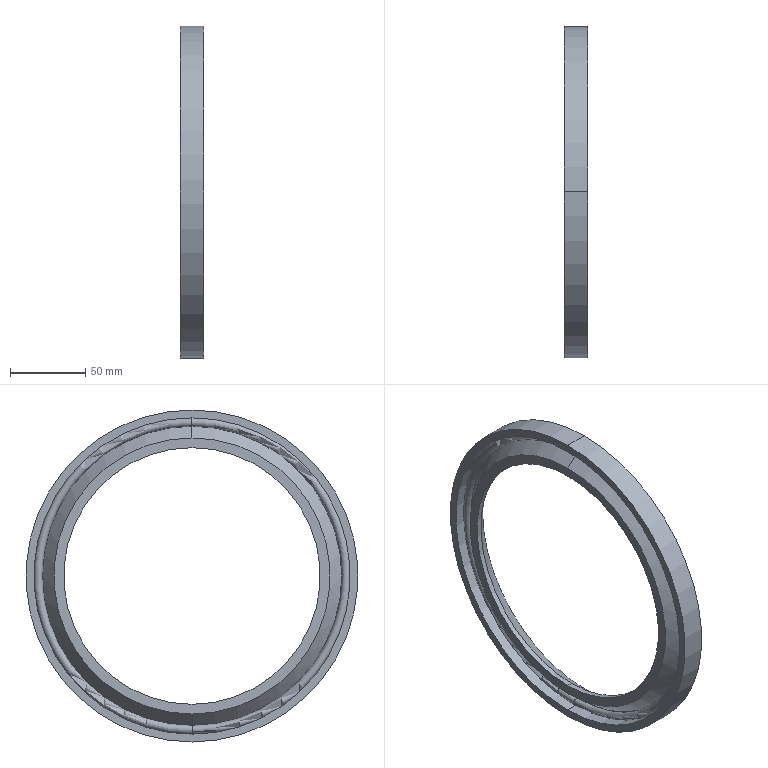Part | STEP file | Seal ring | 2 solids | 19 faces | box 15.499 x 219.997 x 219.997 mm | volume 158146 mm3 | torus 6 | cylinder 6 | cone 4 | plane 3 | commonest cylinder face diameters 170.01 x2 209.598 x2 219.997 x2
STEP:
#1=CARTESIAN_POINT('',(0.,0.,0.));
#2=DIRECTION('',(0.,0.,1.));
#3=DIRECTION('',(1.,0.,0.));
#4=AXIS2_PLACEMENT_3D('',#1,#2,#3);
#5=CARTESIAN_POINT('',(14.065,0.,104.799));
#6=VERTEX_POINT('',#5);
#7=CARTESIAN_POINT('',(14.065,0.,99.229));
#8=VERTEX_POINT('',#7);
#9=CARTESIAN_POINT('',(14.065,0.,102.014));
#10=DIRECTION('',(0.,1.,0.));
#11=DIRECTION('',(0.,0.,1.));
#12=AXIS2_PLACEMENT_3D('',#9,#10,#11);
#13=CIRCLE('',#12,2.785);
#14=CARTESIAN_POINT('',(14.065,0.,0.));
#15=DIRECTION('',(1.,0.,0.));
#16=DIRECTION('',(0.,0.,-1.));
#17=AXIS2_PLACEMENT_3D('',#14,#15,#16);
#18=TOROIDAL_SURFACE('',#17,102.014,2.785);
#19=CARTESIAN_POINT('',(3.142,0.));
#20=DIRECTION('',(0.,1.));
#21=VECTOR('',#20,1.);
#22=LINE('',#19,#21);
#23=(GEOMETRIC_REPRESENTATION_CONTEXT(2)PARAMETRIC_REPRESENTATION_CONTEXT()REPRESENTATION_CONTEXT('',''));
#24=DEFINITIONAL_REPRESENTATION('',(#22),#23);
#25=PCURVE('',#18,#24);
#26=CARTESIAN_POINT('',(14.065,0.,0.));
#27=DIRECTION('',(1.,0.,0.));
#28=DIRECTION('',(0.,0.,-1.));
#29=AXIS2_PLACEMENT_3D('',#26,#27,#28);
#30=TOROIDAL_SURFACE('',#29,102.014,2.785);
#31=CARTESIAN_POINT('',(3.142,0.));
#32=DIRECTION('',(0.,1.));
#33=VECTOR('',#32,1.);
#34=LINE('',#31,#33);
#35=(GEOMETRIC_REPRESENTATION_CONTEXT(2)PARAMETRIC_REPRESENTATION_CONTEXT()REPRESENTATION_CONTEXT('',''));
#36=DEFINITIONAL_REPRESENTATION('',(#34),#35);
#37=PCURVE('',#30,#36);
#38=SURFACE_CURVE('',#13,(#25,#37),.PCURVE_S1.);
#39=EDGE_CURVE('',#6,#8,#38,.T.);
#40=ORIENTED_EDGE('',*,*,#39,.F.);
#41=CARTESIAN_POINT('',(14.065,0.,-104.799));
#42=VERTEX_POINT('',#41);
#43=CARTESIAN_POINT('',(14.065,0.,0.));
#44=DIRECTION('',(1.,0.,0.));
#45=DIRECTION('',(0.,0.,-1.));
#46=AXIS2_PLACEMENT_3D('',#43,#44,#45);
#47=CIRCLE('',#46,104.799);
#48=CARTESIAN_POINT('',(0.,0.));
#49=DIRECTION('',(1.,0.));
#50=VECTOR('',#49,1.);
#51=LINE('',#48,#50);
#52=(GEOMETRIC_REPRESENTATION_CONTEXT(2)PARAMETRIC_REPRESENTATION_CONTEXT()REPRESENTATION_CONTEXT('',''));
#53=DEFINITIONAL_REPRESENTATION('',(#51),#52);
#54=PCURVE('',#18,#53);
#55=CARTESIAN_POINT('',(14.065,0.,0.));
#56=DIRECTION('',(1.,0.,0.));
#57=DIRECTION('',(0.,0.,-1.));
#58=AXIS2_PLACEMENT_3D('',#55,#56,#57);
#59=TOROIDAL_SURFACE('',#58,102.014,2.785);
#60=CARTESIAN_POINT('',(0.,6.283));
#61=DIRECTION('',(1.,0.));
#62=VECTOR('',#61,1.);
#63=LINE('',#60,#62);
#64=(GEOMETRIC_REPRESENTATION_CONTEXT(2)PARAMETRIC_REPRESENTATION_CONTEXT()REPRESENTATION_CONTEXT('',''));
#65=DEFINITIONAL_REPRESENTATION('',(#63),#64);
#66=PCURVE('',#59,#65);
#67=SURFACE_CURVE('',#47,(#54,#66),.PCURVE_S1.);
#68=EDGE_CURVE('',#6,#42,#67,.T.);
#69=ORIENTED_EDGE('',*,*,#68,.T.);
#70=CARTESIAN_POINT('',(14.065,0.,-99.229));
#71=VERTEX_POINT('',#70);
#72=CARTESIAN_POINT('',(14.065,0.,-102.014));
#73=DIRECTION('',(0.,-1.,0.));
#74=DIRECTION('',(0.,0.,-1.));
#75=AXIS2_PLACEMENT_3D('',#72,#73,#74);
#76=CIRCLE('',#75,2.785);
#77=CARTESIAN_POINT('',(6.283,0.));
#78=DIRECTION('',(0.,1.));
#79=VECTOR('',#78,1.);
#80=LINE('',#77,#79);
#81=(GEOMETRIC_REPRESENTATION_CONTEXT(2)PARAMETRIC_REPRESENTATION_CONTEXT()REPRESENTATION_CONTEXT('',''));
#82=DEFINITIONAL_REPRESENTATION('',(#80),#81);
#83=PCURVE('',#18,#82);
#84=CARTESIAN_POINT('',(0.,0.));
#85=DIRECTION('',(0.,1.));
#86=VECTOR('',#85,1.);
#87=LINE('',#84,#86);
#88=(GEOMETRIC_REPRESENTATION_CONTEXT(2)PARAMETRIC_REPRESENTATION_CONTEXT()REPRESENTATION_CONTEXT('',''));
#89=DEFINITIONAL_REPRESENTATION('',(#87),#88);
#90=PCURVE('',#30,#89);
#91=SURFACE_CURVE('',#76,(#83,#90),.PCURVE_S1.);
#92=EDGE_CURVE('',#42,#71,#91,.T.);
#93=ORIENTED_EDGE('',*,*,#92,.T.);
#94=CARTESIAN_POINT('',(14.065,0.,0.));
#95=DIRECTION('',(1.,0.,0.));
#96=DIRECTION('',(0.,0.,-1.));
#97=AXIS2_PLACEMENT_3D('',#94,#95,#96);
#98=CIRCLE('',#97,99.229);
#99=CARTESIAN_POINT('',(0.,3.142));
#100=DIRECTION('',(1.,0.));
#101=VECTOR('',#100,1.);
#102=LINE('',#99,#101);
#103=(GEOMETRIC_REPRESENTATION_CONTEXT(2)PARAMETRIC_REPRESENTATION_CONTEXT()REPRESENTATION_CONTEXT('',''));
#104=DEFINITIONAL_REPRESENTATION('',(#102),#103);
#105=PCURVE('',#18,#104);
#106=CARTESIAN_POINT('',(0.,3.142));
#107=DIRECTION('',(1.,0.));
#108=VECTOR('',#107,1.);
#109=LINE('',#106,#108);
#110=(GEOMETRIC_REPRESENTATION_CONTEXT(2)PARAMETRIC_REPRESENTATION_CONTEXT()REPRESENTATION_CONTEXT('',''));
#111=DEFINITIONAL_REPRESENTATION('',(#109),#110);
#112=PCURVE('',#59,#111);
#113=SURFACE_CURVE('',#98,(#105,#112),.PCURVE_S1.);
#114=EDGE_CURVE('',#8,#71,#113,.T.);
#115=ORIENTED_EDGE('',*,*,#114,.F.);
#116=EDGE_LOOP('',(#40,#69,#93,#115));
#117=FACE_BOUND('',#116,.T.);
#118=ADVANCED_FACE('',(#117),#18,.T.);
#119=ORIENTED_EDGE('',*,*,#92,.F.);
#120=CARTESIAN_POINT('',(14.065,0.,0.));
#121=DIRECTION('',(1.,0.,0.));
#122=DIRECTION('',(0.,0.,-1.));
#123=AXIS2_PLACEMENT_3D('',#120,#121,#122);
#124=CIRCLE('',#123,104.799);
#125=CARTESIAN_POINT('',(0.,0.));
#126=DIRECTION('',(1.,0.));
#127=VECTOR('',#126,1.);
#128=LINE('',#125,#127);
#129=(GEOMETRIC_REPRESENTATION_CONTEXT(2)PARAMETRIC_REPRESENTATION_CONTEXT()REPRESENTATION_CONTEXT('',''));
#130=DEFINITIONAL_REPRESENTATION('',(#128),#129);
#131=PCURVE('',#30,#130);
#132=CARTESIAN_POINT('',(14.065,0.,0.));
#133=DIRECTION('',(1.,0.,0.));
#134=DIRECTION('',(0.,0.,-1.));
#135=AXIS2_PLACEMENT_3D('',#132,#133,#134);
#136=TOROIDAL_SURFACE('',#135,102.014,2.785);
#137=CARTESIAN_POINT('',(0.,6.283));
#138=DIRECTION('',(1.,0.));
#139=VECTOR('',#138,1.);
#140=LINE('',#137,#139);
#141=(GEOMETRIC_REPRESENTATION_CONTEXT(2)PARAMETRIC_REPRESENTATION_CONTEXT()REPRESENTATION_CONTEXT('',''));
#142=DEFINITIONAL_REPRESENTATION('',(#140),#141);
#143=PCURVE('',#136,#142);
#144=SURFACE_CURVE('',#124,(#131,#143),.PCURVE_S1.);
#145=EDGE_CURVE('',#42,#6,#144,.T.);
#146=ORIENTED_EDGE('',*,*,#145,.T.);
#147=ORIENTED_EDGE('',*,*,#39,.T.);
#148=CARTESIAN_POINT('',(14.065,0.,0.));
#149=DIRECTION('',(1.,0.,0.));
#150=DIRECTION('',(0.,0.,-1.));
#151=AXIS2_PLACEMENT_3D('',#148,#149,#150);
#152=CIRCLE('',#151,99.229);
#153=CARTESIAN_POINT('',(0.,3.142));
#154=DIRECTION('',(1.,0.));
#155=VECTOR('',#154,1.);
#156=LINE('',#153,#155);
#157=(GEOMETRIC_REPRESENTATION_CONTEXT(2)PARAMETRIC_REPRESENTATION_CONTEXT()REPRESENTATION_CONTEXT('',''));
#158=DEFINITIONAL_REPRESENTATION('',(#156),#157);
#159=PCURVE('',#30,#158);
#160=CARTESIAN_POINT('',(0.,3.142));
#161=DIRECTION('',(1.,0.));
#162=VECTOR('',#161,1.);
#163=LINE('',#160,#162);
#164=(GEOMETRIC_REPRESENTATION_CONTEXT(2)PARAMETRIC_REPRESENTATION_CONTEXT()REPRESENTATION_CONTEXT('',''));
#165=DEFINITIONAL_REPRESENTATION('',(#163),#164);
#166=PCURVE('',#136,#165);
#167=SURFACE_CURVE('',#152,(#159,#166),.PCURVE_S1.);
#168=EDGE_CURVE('',#71,#8,#167,.T.);
#169=ORIENTED_EDGE('',*,*,#168,.F.);
#170=EDGE_LOOP('',(#119,#146,#147,#169));
#171=FACE_BOUND('',#170,.T.);
#172=ADVANCED_FACE('',(#171),#30,.T.);
#173=ORIENTED_EDGE('',*,*,#145,.F.);
#174=CARTESIAN_POINT('',(14.065,0.,-102.014));
#175=DIRECTION('',(0.,-1.,0.));
#176=DIRECTION('',(0.,0.,-1.));
#177=AXIS2_PLACEMENT_3D('',#174,#175,#176);
#178=CIRCLE('',#177,2.785);
#179=CARTESIAN_POINT('',(0.,0.));
#180=DIRECTION('',(0.,1.));
#181=VECTOR('',#180,1.);
#182=LINE('',#179,#181);
#183=(GEOMETRIC_REPRESENTATION_CONTEXT(2)PARAMETRIC_REPRESENTATION_CONTEXT()REPRESENTATION_CONTEXT('',''));
#184=DEFINITIONAL_REPRESENTATION('',(#182),#183);
#185=PCURVE('',#136,#184);
#186=CARTESIAN_POINT('',(6.283,0.));
#187=DIRECTION('',(0.,1.));
#188=VECTOR('',#187,1.);
#189=LINE('',#186,#188);
#190=(GEOMETRIC_REPRESENTATION_CONTEXT(2)PARAMETRIC_REPRESENTATION_CONTEXT()REPRESENTATION_CONTEXT('',''));
#191=DEFINITIONAL_REPRESENTATION('',(#189),#190);
#192=PCURVE('',#59,#191);
#193=SURFACE_CURVE('',#178,(#185,#192),.PCURVE_S1.);
#194=EDGE_CURVE('',#71,#42,#193,.T.);
#195=ORIENTED_EDGE('',*,*,#194,.F.);
#196=ORIENTED_EDGE('',*,*,#168,.T.);
#197=CARTESIAN_POINT('',(14.065,0.,102.014));
#198=DIRECTION('',(0.,1.,0.));
#199=DIRECTION('',(0.,0.,1.));
#200=AXIS2_PLACEMENT_3D('',#197,#198,#199);
#201=CIRCLE('',#200,2.785);
#202=CARTESIAN_POINT('',(3.142,0.));
#203=DIRECTION('',(0.,1.));
#204=VECTOR('',#203,1.);
#205=LINE('',#202,#204);
#206=(GEOMETRIC_REPRESENTATION_CONTEXT(2)PARAMETRIC_REPRESENTATION_CONTEXT()REPRESENTATION_CONTEXT('',''));
#207=DEFINITIONAL_REPRESENTATION('',(#205),#206);
#208=PCURVE('',#136,#207);
#209=CARTESIAN_POINT('',(3.142,0.));
#210=DIRECTION('',(0.,1.));
#211=VECTOR('',#210,1.);
#212=LINE('',#209,#211);
#213=(GEOMETRIC_REPRESENTATION_CONTEXT(2)PARAMETRIC_REPRESENTATION_CONTEXT()REPRESENTATION_CONTEXT('',''));
#214=DEFINITIONAL_REPRESENTATION('',(#212),#213);
#215=PCURVE('',#59,#214);
#216=SURFACE_CURVE('',#201,(#208,#215),.PCURVE_S1.);
#217=EDGE_CURVE('',#8,#6,#216,.T.);
#218=ORIENTED_EDGE('',*,*,#217,.T.);
#219=EDGE_LOOP('',(#173,#195,#196,#218));
#220=FACE_BOUND('',#219,.T.);
#221=ADVANCED_FACE('',(#220),#136,.T.);
#222=ORIENTED_EDGE('',*,*,#68,.F.);
#223=ORIENTED_EDGE('',*,*,#217,.F.);
#224=ORIENTED_EDGE('',*,*,#114,.T.);
#225=ORIENTED_EDGE('',*,*,#194,.T.);
#226=EDGE_LOOP('',(#222,#223,#224,#225));
#227=FACE_BOUND('',#226,.T.);
#228=ADVANCED_FACE('',(#227),#59,.T.);
#229=CLOSED_SHELL('',(#118,#172,#221,#228));
#230=MANIFOLD_SOLID_BREP('',#229);
#231=CARTESIAN_POINT('',(5.58,0.,-104.799));
#232=VERTEX_POINT('',#231);
#233=CARTESIAN_POINT('',(14.065,0.,-104.799));
#234=VERTEX_POINT('',#233);
#235=CARTESIAN_POINT('',(0.,0.,-104.799));
#236=DIRECTION('',(1.,0.,0.));
#237=VECTOR('',#236,1.);
#238=LINE('',#235,#237);
#239=CARTESIAN_POINT('',(0.,0.,0.));
#240=DIRECTION('',(1.,0.,0.));
#241=DIRECTION('',(0.,0.,-1.));
#242=AXIS2_PLACEMENT_3D('',#239,#240,#241);
#243=CYLINDRICAL_SURFACE('',#242,104.799);
#244=CARTESIAN_POINT('',(6.283,0.));
#245=DIRECTION('',(0.,1.));
#246=VECTOR('',#245,1.);
#247=LINE('',#244,#246);
#248=(GEOMETRIC_REPRESENTATION_CONTEXT(2)PARAMETRIC_REPRESENTATION_CONTEXT()REPRESENTATION_CONTEXT('',''));
#249=DEFINITIONAL_REPRESENTATION('',(#247),#248);
#250=PCURVE('',#243,#249);
#251=CARTESIAN_POINT('',(0.,0.,0.));
#252=DIRECTION('',(1.,0.,0.));
#253=DIRECTION('',(0.,0.,-1.));
#254=AXIS2_PLACEMENT_3D('',#251,#252,#253);
#255=CYLINDRICAL_SURFACE('',#254,104.799);
#256=CARTESIAN_POINT('',(0.,0.));
#257=DIRECTION('',(0.,1.));
#258=VECTOR('',#257,1.);
#259=LINE('',#256,#258);
#260=(GEOMETRIC_REPRESENTATION_CONTEXT(2)PARAMETRIC_REPRESENTATION_CONTEXT()REPRESENTATION_CONTEXT('',''));
#261=DEFINITIONAL_REPRESENTATION('',(#259),#260);
#262=PCURVE('',#255,#261);
#263=SURFACE_CURVE('',#238,(#250,#262),.PCURVE_S1.);
#264=EDGE_CURVE('',#232,#234,#263,.T.);
#265=ORIENTED_EDGE('',*,*,#264,.T.);
#266=CARTESIAN_POINT('',(14.065,0.,104.799));
#267=VERTEX_POINT('',#266);
#268=CARTESIAN_POINT('',(14.065,0.,0.));
#269=DIRECTION('',(1.,0.,0.));
#270=DIRECTION('',(0.,0.,-1.));
#271=AXIS2_PLACEMENT_3D('',#268,#269,#270);
#272=CIRCLE('',#271,104.799);
#273=CARTESIAN_POINT('',(0.,14.065));
#274=DIRECTION('',(1.,0.));
#275=VECTOR('',#274,1.);
#276=LINE('',#273,#275);
#277=(GEOMETRIC_REPRESENTATION_CONTEXT(2)PARAMETRIC_REPRESENTATION_CONTEXT()REPRESENTATION_CONTEXT('',''));
#278=DEFINITIONAL_REPRESENTATION('',(#276),#277);
#279=PCURVE('',#243,#278);
#280=CARTESIAN_POINT('',(14.065,0.,0.));
#281=DIRECTION('',(1.,0.,0.));
#282=DIRECTION('',(0.,0.,-1.));
#283=AXIS2_PLACEMENT_3D('',#280,#281,#282);
#284=TOROIDAL_SURFACE('',#283,102.014,2.785);
#285=CARTESIAN_POINT('',(0.,0.));
#286=DIRECTION('',(1.,0.));
#287=VECTOR('',#286,1.);
#288=LINE('',#285,#287);
#289=(GEOMETRIC_REPRESENTATION_CONTEXT(2)PARAMETRIC_REPRESENTATION_CONTEXT()REPRESENTATION_CONTEXT('',''));
#290=DEFINITIONAL_REPRESENTATION('',(#288),#289);
#291=PCURVE('',#284,#290);
#292=SURFACE_CURVE('',#272,(#279,#291),.PCURVE_S1.);
#293=EDGE_CURVE('',#267,#234,#292,.T.);
#294=ORIENTED_EDGE('',*,*,#293,.F.);
#295=CARTESIAN_POINT('',(5.58,0.,104.799));
#296=VERTEX_POINT('',#295);
#297=CARTESIAN_POINT('',(0.,0.,104.799));
#298=DIRECTION('',(1.,0.,0.));
#299=VECTOR('',#298,1.);
#300=LINE('',#297,#299);
#301=CARTESIAN_POINT('',(3.142,0.));
#302=DIRECTION('',(0.,1.));
#303=VECTOR('',#302,1.);
#304=LINE('',#301,#303);
#305=(GEOMETRIC_REPRESENTATION_CONTEXT(2)PARAMETRIC_REPRESENTATION_CONTEXT()REPRESENTATION_CONTEXT('',''));
#306=DEFINITIONAL_REPRESENTATION('',(#304),#305);
#307=PCURVE('',#243,#306);
#308=CARTESIAN_POINT('',(3.142,0.));
#309=DIRECTION('',(0.,1.));
#310=VECTOR('',#309,1.);
#311=LINE('',#308,#310);
#312=(GEOMETRIC_REPRESENTATION_CONTEXT(2)PARAMETRIC_REPRESENTATION_CONTEXT()REPRESENTATION_CONTEXT('',''));
#313=DEFINITIONAL_REPRESENTATION('',(#311),#312);
#314=PCURVE('',#255,#313);
#315=SURFACE_CURVE('',#300,(#307,#314),.PCURVE_S1.);
#316=EDGE_CURVE('',#296,#267,#315,.T.);
#317=ORIENTED_EDGE('',*,*,#316,.F.);
#318=CARTESIAN_POINT('',(5.58,0.,0.));
#319=DIRECTION('',(1.,0.,0.));
#320=DIRECTION('',(0.,0.,-1.));
#321=AXIS2_PLACEMENT_3D('',#318,#319,#320);
#322=CIRCLE('',#321,104.799);
#323=CARTESIAN_POINT('',(0.,5.58));
#324=DIRECTION('',(1.,0.));
#325=VECTOR('',#324,1.);
#326=LINE('',#323,#325);
#327=(GEOMETRIC_REPRESENTATION_CONTEXT(2)PARAMETRIC_REPRESENTATION_CONTEXT()REPRESENTATION_CONTEXT('',''));
#328=DEFINITIONAL_REPRESENTATION('',(#326),#327);
#329=PCURVE('',#243,#328);
#330=CARTESIAN_POINT('',(5.58,0.,0.));
#331=DIRECTION('',(-1.,0.,0.));
#332=DIRECTION('',(0.,0.,1.));
#333=AXIS2_PLACEMENT_3D('',#330,#331,#332);
#334=PLANE('',#333);
#335=CARTESIAN_POINT('',(-104.799,0.));
#336=CARTESIAN_POINT('',(-104.799,181.517));
#337=CARTESIAN_POINT('',(52.399,90.759));
#338=CARTESIAN_POINT('',(209.598,0.));
#339=CARTESIAN_POINT('',(52.399,-90.759));
#340=CARTESIAN_POINT('',(-104.799,-181.517));
#341=CARTESIAN_POINT('',(-104.799,0.));
#342=(BOUNDED_CURVE()B_SPLINE_CURVE(2,(#335,#336,#337,#338,#339,#340,#341),.UNSPECIFIED.,.T.,.F.)B_SPLINE_CURVE_WITH_KNOTS((1,2,2,2,2,1),(-2.094,0.,2.094,4.189,6.283,8.378),.UNSPECIFIED.)CURVE()GEOMETRIC_REPRESENTATION_ITEM()RATIONAL_B_SPLINE_CURVE((1.,0.5,1.,0.5,1.,0.5,1.))REPRESENTATION_ITEM(''));
#343=(GEOMETRIC_REPRESENTATION_CONTEXT(2)PARAMETRIC_REPRESENTATION_CONTEXT()REPRESENTATION_CONTEXT('',''));
#344=DEFINITIONAL_REPRESENTATION('',(#342),#343);
#345=PCURVE('',#334,#344);
#346=SURFACE_CURVE('',#322,(#329,#345),.PCURVE_S1.);
#347=EDGE_CURVE('',#296,#232,#346,.T.);
#348=ORIENTED_EDGE('',*,*,#347,.T.);
#349=EDGE_LOOP('',(#265,#294,#317,#348));
#350=FACE_BOUND('',#349,.F.);
#351=ADVANCED_FACE('',(#350),#243,.F.);
#352=CARTESIAN_POINT('',(5.58,0.,-109.999));
#353=VERTEX_POINT('',#352);
#354=CARTESIAN_POINT('',(5.58,0.,109.999));
#355=VERTEX_POINT('',#354);
#356=CARTESIAN_POINT('',(5.58,0.,0.));
#357=DIRECTION('',(1.,0.,0.));
#358=DIRECTION('',(0.,0.,-1.));
#359=AXIS2_PLACEMENT_3D('',#356,#357,#358);
#360=CIRCLE('',#359,109.999);
#361=CARTESIAN_POINT('',(0.,0.,0.));
#362=DIRECTION('',(1.,0.,0.));
#363=DIRECTION('',(0.,0.,-1.));
#364=AXIS2_PLACEMENT_3D('',#361,#362,#363);
#365=CYLINDRICAL_SURFACE('',#364,109.999);
#366=CARTESIAN_POINT('',(0.,5.58));
#367=DIRECTION('',(1.,0.));
#368=VECTOR('',#367,1.);
#369=LINE('',#366,#368);
#370=(GEOMETRIC_REPRESENTATION_CONTEXT(2)PARAMETRIC_REPRESENTATION_CONTEXT()REPRESENTATION_CONTEXT('',''));
#371=DEFINITIONAL_REPRESENTATION('',(#369),#370);
#372=PCURVE('',#365,#371);
#373=CARTESIAN_POINT('',(-109.999,0.));
#374=CARTESIAN_POINT('',(-109.999,190.523));
#375=CARTESIAN_POINT('',(54.999,95.262));
#376=CARTESIAN_POINT('',(219.997,0.));
#377=CARTESIAN_POINT('',(54.999,-95.262));
#378=CARTESIAN_POINT('',(-109.999,-190.523));
#379=CARTESIAN_POINT('',(-109.999,0.));
#380=(BOUNDED_CURVE()B_SPLINE_CURVE(2,(#373,#374,#375,#376,#377,#378,#379),.UNSPECIFIED.,.T.,.F.)B_SPLINE_CURVE_WITH_KNOTS((1,2,2,2,2,1),(-2.094,0.,2.094,4.189,6.283,8.378),.UNSPECIFIED.)CURVE()GEOMETRIC_REPRESENTATION_ITEM()RATIONAL_B_SPLINE_CURVE((1.,0.5,1.,0.5,1.,0.5,1.))REPRESENTATION_ITEM(''));
#381=(GEOMETRIC_REPRESENTATION_CONTEXT(2)PARAMETRIC_REPRESENTATION_CONTEXT()REPRESENTATION_CONTEXT('',''));
#382=DEFINITIONAL_REPRESENTATION('',(#380),#381);
#383=PCURVE('',#334,#382);
#384=SURFACE_CURVE('',#360,(#372,#383),.PCURVE_S1.);
#385=EDGE_CURVE('',#353,#355,#384,.T.);
#386=ORIENTED_EDGE('',*,*,#385,.T.);
#387=CARTESIAN_POINT('',(21.079,0.,109.999));
#388=VERTEX_POINT('',#387);
#389=CARTESIAN_POINT('',(0.,0.,109.999));
#390=DIRECTION('',(1.,0.,0.));
#391=VECTOR('',#390,1.);
#392=LINE('',#389,#391);
#393=CARTESIAN_POINT('',(3.142,0.));
#394=DIRECTION('',(0.,1.));
#395=VECTOR('',#394,1.);
#396=LINE('',#393,#395);
#397=(GEOMETRIC_REPRESENTATION_CONTEXT(2)PARAMETRIC_REPRESENTATION_CONTEXT()REPRESENTATION_CONTEXT('',''));
#398=DEFINITIONAL_REPRESENTATION('',(#396),#397);
#399=PCURVE('',#365,#398);
#400=CARTESIAN_POINT('',(0.,0.,0.));
#401=DIRECTION('',(1.,0.,0.));
#402=DIRECTION('',(0.,0.,-1.));
#403=AXIS2_PLACEMENT_3D('',#400,#401,#402);
#404=CYLINDRICAL_SURFACE('',#403,109.999);
#405=CARTESIAN_POINT('',(3.142,0.));
#406=DIRECTION('',(0.,1.));
#407=VECTOR('',#406,1.);
#408=LINE('',#405,#407);
#409=(GEOMETRIC_REPRESENTATION_CONTEXT(2)PARAMETRIC_REPRESENTATION_CONTEXT()REPRESENTATION_CONTEXT('',''));
#410=DEFINITIONAL_REPRESENTATION('',(#408),#409);
#411=PCURVE('',#404,#410);
#412=SURFACE_CURVE('',#392,(#399,#411),.PCURVE_S1.);
#413=EDGE_CURVE('',#355,#388,#412,.T.);
#414=ORIENTED_EDGE('',*,*,#413,.T.);
#415=CARTESIAN_POINT('',(21.079,0.,-109.999));
#416=VERTEX_POINT('',#415);
#417=CARTESIAN_POINT('',(21.079,0.,0.));
#418=DIRECTION('',(1.,0.,0.));
#419=DIRECTION('',(0.,0.,-1.));
#420=AXIS2_PLACEMENT_3D('',#417,#418,#419);
#421=CIRCLE('',#420,109.999);
#422=CARTESIAN_POINT('',(0.,21.079));
#423=DIRECTION('',(1.,0.));
#424=VECTOR('',#423,1.);
#425=LINE('',#422,#424);
#426=(GEOMETRIC_REPRESENTATION_CONTEXT(2)PARAMETRIC_REPRESENTATION_CONTEXT()REPRESENTATION_CONTEXT('',''));
#427=DEFINITIONAL_REPRESENTATION('',(#425),#426);
#428=PCURVE('',#365,#427);
#429=CARTESIAN_POINT('',(21.079,0.,0.));
#430=DIRECTION('',(-1.,0.,0.));
#431=DIRECTION('',(0.,0.,1.));
#432=AXIS2_PLACEMENT_3D('',#429,#430,#431);
#433=PLANE('',#432);
#434=CARTESIAN_POINT('',(-109.999,0.));
#435=CARTESIAN_POINT('',(-109.999,190.523));
#436=CARTESIAN_POINT('',(54.999,95.262));
#437=CARTESIAN_POINT('',(219.997,0.));
#438=CARTESIAN_POINT('',(54.999,-95.262));
#439=CARTESIAN_POINT('',(-109.999,-190.523));
#440=CARTESIAN_POINT('',(-109.999,0.));
#441=(BOUNDED_CURVE()B_SPLINE_CURVE(2,(#434,#435,#436,#437,#438,#439,#440),.UNSPECIFIED.,.T.,.F.)B_SPLINE_CURVE_WITH_KNOTS((1,2,2,2,2,1),(-2.094,0.,2.094,4.189,6.283,8.378),.UNSPECIFIED.)CURVE()GEOMETRIC_REPRESENTATION_ITEM()RATIONAL_B_SPLINE_CURVE((1.,0.5,1.,0.5,1.,0.5,1.))REPRESENTATION_ITEM(''));
#442=(GEOMETRIC_REPRESENTATION_CONTEXT(2)PARAMETRIC_REPRESENTATION_CONTEXT()REPRESENTATION_CONTEXT('',''));
#443=DEFINITIONAL_REPRESENTATION('',(#441),#442);
#444=PCURVE('',#433,#443);
#445=SURFACE_CURVE('',#421,(#428,#444),.PCURVE_S1.);
#446=EDGE_CURVE('',#416,#388,#445,.T.);
#447=ORIENTED_EDGE('',*,*,#446,.F.);
#448=CARTESIAN_POINT('',(0.,0.,-109.999));
#449=DIRECTION('',(1.,0.,0.));
#450=VECTOR('',#449,1.);
#451=LINE('',#448,#450);
#452=CARTESIAN_POINT('',(0.,0.));
#453=DIRECTION('',(0.,1.));
#454=VECTOR('',#453,1.);
#455=LINE('',#452,#454);
#456=(GEOMETRIC_REPRESENTATION_CONTEXT(2)PARAMETRIC_REPRESENTATION_CONTEXT()REPRESENTATION_CONTEXT('',''));
#457=DEFINITIONAL_REPRESENTATION('',(#455),#456);
#458=PCURVE('',#365,#457);
#459=CARTESIAN_POINT('',(6.283,0.));
#460=DIRECTION('',(0.,1.));
#461=VECTOR('',#460,1.);
#462=LINE('',#459,#461);
#463=(GEOMETRIC_REPRESENTATION_CONTEXT(2)PARAMETRIC_REPRESENTATION_CONTEXT()REPRESENTATION_CONTEXT('',''));
#464=DEFINITIONAL_REPRESENTATION('',(#462),#463);
#465=PCURVE('',#404,#464);
#466=SURFACE_CURVE('',#451,(#458,#465),.PCURVE_S1.);
#467=EDGE_CURVE('',#353,#416,#466,.T.);
#468=ORIENTED_EDGE('',*,*,#467,.F.);
#469=EDGE_LOOP('',(#386,#414,#447,#468));
#470=FACE_BOUND('',#469,.T.);
#471=ADVANCED_FACE('',(#470),#365,.T.);
#472=CARTESIAN_POINT('',(9.062,0.,-85.005));
#473=VERTEX_POINT('',#472);
#474=CARTESIAN_POINT('',(21.079,0.,-95.297));
#475=VERTEX_POINT('',#474);
#476=CARTESIAN_POINT('',(21.079,0.,-95.297));
#477=DIRECTION('',(0.7595,0.,-0.6505));
#478=VECTOR('',#477,1.);
#479=LINE('',#476,#478);
#480=CARTESIAN_POINT('',(21.079,0.,0.));
#481=DIRECTION('',(1.,0.,0.));
#482=DIRECTION('',(0.,0.,-1.));
#483=AXIS2_PLACEMENT_3D('',#480,#481,#482);
#484=CONICAL_SURFACE('',#483,95.297,0.7082);
#485=CARTESIAN_POINT('',(6.283,0.));
#486=DIRECTION('',(0.,1.));
#487=VECTOR('',#486,1.);
#488=LINE('',#485,#487);
#489=(GEOMETRIC_REPRESENTATION_CONTEXT(2)PARAMETRIC_REPRESENTATION_CONTEXT()REPRESENTATION_CONTEXT('',''));
#490=DEFINITIONAL_REPRESENTATION('',(#488),#489);
#491=PCURVE('',#484,#490);
#492=CARTESIAN_POINT('',(21.079,0.,0.));
#493=DIRECTION('',(1.,0.,0.));
#494=DIRECTION('',(0.,0.,-1.));
#495=AXIS2_PLACEMENT_3D('',#492,#493,#494);
#496=CONICAL_SURFACE('',#495,95.297,0.7082);
#497=CARTESIAN_POINT('',(0.,0.));
#498=DIRECTION('',(0.,1.));
#499=VECTOR('',#498,1.);
#500=LINE('',#497,#499);
#501=(GEOMETRIC_REPRESENTATION_CONTEXT(2)PARAMETRIC_REPRESENTATION_CONTEXT()REPRESENTATION_CONTEXT('',''));
#502=DEFINITIONAL_REPRESENTATION('',(#500),#501);
#503=PCURVE('',#496,#502);
#504=SURFACE_CURVE('',#479,(#491,#503),.PCURVE_S1.);
#505=EDGE_CURVE('',#473,#475,#504,.T.);
#506=ORIENTED_EDGE('',*,*,#505,.T.);
#507=CARTESIAN_POINT('',(21.079,0.,95.297));
#508=VERTEX_POINT('',#507);
#509=CARTESIAN_POINT('',(21.079,0.,0.));
#510=DIRECTION('',(1.,0.,0.));
#511=DIRECTION('',(0.,0.,-1.));
#512=AXIS2_PLACEMENT_3D('',#509,#510,#511);
#513=CIRCLE('',#512,95.297);
#514=CARTESIAN_POINT('',(0.,0.));
#515=DIRECTION('',(1.,0.));
#516=VECTOR('',#515,1.);
#517=LINE('',#514,#516);
#518=(GEOMETRIC_REPRESENTATION_CONTEXT(2)PARAMETRIC_REPRESENTATION_CONTEXT()REPRESENTATION_CONTEXT('',''));
#519=DEFINITIONAL_REPRESENTATION('',(#517),#518);
#520=PCURVE('',#484,#519);
#521=CARTESIAN_POINT('',(-95.297,0.));
#522=CARTESIAN_POINT('',(-95.297,165.059));
#523=CARTESIAN_POINT('',(47.648,82.529));
#524=CARTESIAN_POINT('',(190.594,0.));
#525=CARTESIAN_POINT('',(47.648,-82.529));
#526=CARTESIAN_POINT('',(-95.297,-165.059));
#527=CARTESIAN_POINT('',(-95.297,0.));
#528=(BOUNDED_CURVE()B_SPLINE_CURVE(2,(#521,#522,#523,#524,#525,#526,#527),.UNSPECIFIED.,.T.,.F.)B_SPLINE_CURVE_WITH_KNOTS((1,2,2,2,2,1),(-2.094,0.,2.094,4.189,6.283,8.378),.UNSPECIFIED.)CURVE()GEOMETRIC_REPRESENTATION_ITEM()RATIONAL_B_SPLINE_CURVE((1.,0.5,1.,0.5,1.,0.5,1.))REPRESENTATION_ITEM(''));
#529=(GEOMETRIC_REPRESENTATION_CONTEXT(2)PARAMETRIC_REPRESENTATION_CONTEXT()REPRESENTATION_CONTEXT('',''));
#530=DEFINITIONAL_REPRESENTATION('',(#528),#529);
#531=PCURVE('',#433,#530);
#532=SURFACE_CURVE('',#513,(#520,#531),.PCURVE_S1.);
#533=EDGE_CURVE('',#508,#475,#532,.T.);
#534=ORIENTED_EDGE('',*,*,#533,.F.);
#535=CARTESIAN_POINT('',(9.062,0.,85.005));
#536=VERTEX_POINT('',#535);
#537=CARTESIAN_POINT('',(21.079,0.,95.297));
#538=DIRECTION('',(0.7595,0.,0.6505));
#539=VECTOR('',#538,1.);
#540=LINE('',#537,#539);
#541=CARTESIAN_POINT('',(3.142,0.));
#542=DIRECTION('',(0.,1.));
#543=VECTOR('',#542,1.);
#544=LINE('',#541,#543);
#545=(GEOMETRIC_REPRESENTATION_CONTEXT(2)PARAMETRIC_REPRESENTATION_CONTEXT()REPRESENTATION_CONTEXT('',''));
#546=DEFINITIONAL_REPRESENTATION('',(#544),#545);
#547=PCURVE('',#484,#546);
#548=CARTESIAN_POINT('',(3.142,0.));
#549=DIRECTION('',(0.,1.));
#550=VECTOR('',#549,1.);
#551=LINE('',#548,#550);
#552=(GEOMETRIC_REPRESENTATION_CONTEXT(2)PARAMETRIC_REPRESENTATION_CONTEXT()REPRESENTATION_CONTEXT('',''));
#553=DEFINITIONAL_REPRESENTATION('',(#551),#552);
#554=PCURVE('',#496,#553);
#555=SURFACE_CURVE('',#540,(#547,#554),.PCURVE_S1.);
#556=EDGE_CURVE('',#536,#508,#555,.T.);
#557=ORIENTED_EDGE('',*,*,#556,.F.);
#558=CARTESIAN_POINT('',(9.062,0.,0.));
#559=DIRECTION('',(1.,0.,0.));
#560=DIRECTION('',(0.,0.,-1.));
#561=AXIS2_PLACEMENT_3D('',#558,#559,#560);
#562=CIRCLE('',#561,85.005);
#563=CARTESIAN_POINT('',(0.,-12.017));
#564=DIRECTION('',(1.,0.));
#565=VECTOR('',#564,1.);
#566=LINE('',#563,#565);
#567=(GEOMETRIC_REPRESENTATION_CONTEXT(2)PARAMETRIC_REPRESENTATION_CONTEXT()REPRESENTATION_CONTEXT('',''));
#568=DEFINITIONAL_REPRESENTATION('',(#566),#567);
#569=PCURVE('',#484,#568);
#570=CARTESIAN_POINT('',(0.,0.,0.));
#571=DIRECTION('',(1.,0.,0.));
#572=DIRECTION('',(0.,0.,-1.));
#573=AXIS2_PLACEMENT_3D('',#570,#571,#572);
#574=CYLINDRICAL_SURFACE('',#573,85.005);
#575=CARTESIAN_POINT('',(0.,9.062));
#576=DIRECTION('',(1.,0.));
#577=VECTOR('',#576,1.);
#578=LINE('',#575,#577);
#579=(GEOMETRIC_REPRESENTATION_CONTEXT(2)PARAMETRIC_REPRESENTATION_CONTEXT()REPRESENTATION_CONTEXT('',''));
#580=DEFINITIONAL_REPRESENTATION('',(#578),#579);
#581=PCURVE('',#574,#580);
#582=SURFACE_CURVE('',#562,(#569,#581),.PCURVE_S1.);
#583=EDGE_CURVE('',#536,#473,#582,.T.);
#584=ORIENTED_EDGE('',*,*,#583,.T.);
#585=EDGE_LOOP('',(#506,#534,#557,#584));
#586=FACE_BOUND('',#585,.F.);
#587=ADVANCED_FACE('',(#586),#484,.F.);
#588=CARTESIAN_POINT('',(5.583,0.,-85.005));
#589=VERTEX_POINT('',#588);
#590=CARTESIAN_POINT('',(0.,0.,-85.005));
#591=DIRECTION('',(1.,0.,0.));
#592=VECTOR('',#591,1.);
#593=LINE('',#590,#592);
#594=CARTESIAN_POINT('',(6.283,0.));
#595=DIRECTION('',(0.,1.));
#596=VECTOR('',#595,1.);
#597=LINE('',#594,#596);
#598=(GEOMETRIC_REPRESENTATION_CONTEXT(2)PARAMETRIC_REPRESENTATION_CONTEXT()REPRESENTATION_CONTEXT('',''));
#599=DEFINITIONAL_REPRESENTATION('',(#597),#598);
#600=PCURVE('',#574,#599);
#601=CARTESIAN_POINT('',(0.,0.,0.));
#602=DIRECTION('',(1.,0.,0.));
#603=DIRECTION('',(0.,0.,-1.));
#604=AXIS2_PLACEMENT_3D('',#601,#602,#603);
#605=CYLINDRICAL_SURFACE('',#604,85.005);
#606=CARTESIAN_POINT('',(0.,0.));
#607=DIRECTION('',(0.,1.));
#608=VECTOR('',#607,1.);
#609=LINE('',#606,#608);
#610=(GEOMETRIC_REPRESENTATION_CONTEXT(2)PARAMETRIC_REPRESENTATION_CONTEXT()REPRESENTATION_CONTEXT('',''));
#611=DEFINITIONAL_REPRESENTATION('',(#609),#610);
#612=PCURVE('',#605,#611);
#613=SURFACE_CURVE('',#593,(#600,#612),.PCURVE_S1.);
#614=EDGE_CURVE('',#589,#473,#613,.T.);
#615=ORIENTED_EDGE('',*,*,#614,.T.);
#616=ORIENTED_EDGE('',*,*,#583,.F.);
#617=CARTESIAN_POINT('',(5.583,0.,85.005));
#618=VERTEX_POINT('',#617);
#619=CARTESIAN_POINT('',(0.,0.,85.005));
#620=DIRECTION('',(1.,0.,0.));
#621=VECTOR('',#620,1.);
#622=LINE('',#619,#621);
#623=CARTESIAN_POINT('',(3.142,0.));
#624=DIRECTION('',(0.,1.));
#625=VECTOR('',#624,1.);
#626=LINE('',#623,#625);
#627=(GEOMETRIC_REPRESENTATION_CONTEXT(2)PARAMETRIC_REPRESENTATION_CONTEXT()REPRESENTATION_CONTEXT('',''));
#628=DEFINITIONAL_REPRESENTATION('',(#626),#627);
#629=PCURVE('',#574,#628);
#630=CARTESIAN_POINT('',(3.142,0.));
#631=DIRECTION('',(0.,1.));
#632=VECTOR('',#631,1.);
#633=LINE('',#630,#632);
#634=(GEOMETRIC_REPRESENTATION_CONTEXT(2)PARAMETRIC_REPRESENTATION_CONTEXT()REPRESENTATION_CONTEXT('',''));
#635=DEFINITIONAL_REPRESENTATION('',(#633),#634);
#636=PCURVE('',#605,#635);
#637=SURFACE_CURVE('',#622,(#629,#636),.PCURVE_S1.);
#638=EDGE_CURVE('',#618,#536,#637,.T.);
#639=ORIENTED_EDGE('',*,*,#638,.F.);
#640=CARTESIAN_POINT('',(5.583,0.,0.));
#641=DIRECTION('',(1.,0.,0.));
#642=DIRECTION('',(0.,0.,-1.));
#643=AXIS2_PLACEMENT_3D('',#640,#641,#642);
#644=CIRCLE('',#643,85.005);
#645=CARTESIAN_POINT('',(0.,5.583));
#646=DIRECTION('',(1.,0.));
#647=VECTOR('',#646,1.);
#648=LINE('',#645,#647);
#649=(GEOMETRIC_REPRESENTATION_CONTEXT(2)PARAMETRIC_REPRESENTATION_CONTEXT()REPRESENTATION_CONTEXT('',''));
#650=DEFINITIONAL_REPRESENTATION('',(#648),#649);
#651=PCURVE('',#574,#650);
#652=CARTESIAN_POINT('',(5.583,0.,0.));
#653=DIRECTION('',(-1.,0.,0.));
#654=DIRECTION('',(0.,0.,1.));
#655=AXIS2_PLACEMENT_3D('',#652,#653,#654);
#656=PLANE('',#655);
#657=CARTESIAN_POINT('',(-85.005,0.));
#658=CARTESIAN_POINT('',(-85.005,147.233));
#659=CARTESIAN_POINT('',(42.502,73.616));
#660=CARTESIAN_POINT('',(170.01,0.));
#661=CARTESIAN_POINT('',(42.502,-73.616));
#662=CARTESIAN_POINT('',(-85.005,-147.233));
#663=CARTESIAN_POINT('',(-85.005,0.));
#664=(BOUNDED_CURVE()B_SPLINE_CURVE(2,(#657,#658,#659,#660,#661,#662,#663),.UNSPECIFIED.,.T.,.F.)B_SPLINE_CURVE_WITH_KNOTS((1,2,2,2,2,1),(-2.094,0.,2.094,4.189,6.283,8.378),.UNSPECIFIED.)CURVE()GEOMETRIC_REPRESENTATION_ITEM()RATIONAL_B_SPLINE_CURVE((1.,0.5,1.,0.5,1.,0.5,1.))REPRESENTATION_ITEM(''));
#665=(GEOMETRIC_REPRESENTATION_CONTEXT(2)PARAMETRIC_REPRESENTATION_CONTEXT()REPRESENTATION_CONTEXT('',''));
#666=DEFINITIONAL_REPRESENTATION('',(#664),#665);
#667=PCURVE('',#656,#666);
#668=SURFACE_CURVE('',#644,(#651,#667),.PCURVE_S1.);
#669=EDGE_CURVE('',#618,#589,#668,.T.);
#670=ORIENTED_EDGE('',*,*,#669,.T.);
#671=EDGE_LOOP('',(#615,#616,#639,#670));
#672=FACE_BOUND('',#671,.F.);
#673=ADVANCED_FACE('',(#672),#574,.F.);
#674=CARTESIAN_POINT('',(5.583,0.,-91.5));
#675=VERTEX_POINT('',#674);
#676=CARTESIAN_POINT('',(5.583,0.,91.5));
#677=VERTEX_POINT('',#676);
#678=CARTESIAN_POINT('',(5.583,0.,0.));
#679=DIRECTION('',(1.,0.,0.));
#680=DIRECTION('',(0.,0.,-1.));
#681=AXIS2_PLACEMENT_3D('',#678,#679,#680);
#682=CIRCLE('',#681,91.5);
#683=CARTESIAN_POINT('',(15.826,0.,0.));
#684=DIRECTION('',(1.,0.,0.));
#685=DIRECTION('',(0.,0.,-1.));
#686=AXIS2_PLACEMENT_3D('',#683,#684,#685);
#687=CONICAL_SURFACE('',#686,99.856,0.6843);
#688=CARTESIAN_POINT('',(0.,-10.243));
#689=DIRECTION('',(1.,0.));
#690=VECTOR('',#689,1.);
#691=LINE('',#688,#690);
#692=(GEOMETRIC_REPRESENTATION_CONTEXT(2)PARAMETRIC_REPRESENTATION_CONTEXT()REPRESENTATION_CONTEXT('',''));
#693=DEFINITIONAL_REPRESENTATION('',(#691),#692);
#694=PCURVE('',#687,#693);
#695=CARTESIAN_POINT('',(-91.5,0.));
#696=CARTESIAN_POINT('',(-91.5,158.483));
#697=CARTESIAN_POINT('',(45.75,79.241));
#698=CARTESIAN_POINT('',(183.,0.));
#699=CARTESIAN_POINT('',(45.75,-79.241));
#700=CARTESIAN_POINT('',(-91.5,-158.483));
#701=CARTESIAN_POINT('',(-91.5,0.));
#702=(BOUNDED_CURVE()B_SPLINE_CURVE(2,(#695,#696,#697,#698,#699,#700,#701),.UNSPECIFIED.,.T.,.F.)B_SPLINE_CURVE_WITH_KNOTS((1,2,2,2,2,1),(-2.094,0.,2.094,4.189,6.283,8.378),.UNSPECIFIED.)CURVE()GEOMETRIC_REPRESENTATION_ITEM()RATIONAL_B_SPLINE_CURVE((1.,0.5,1.,0.5,1.,0.5,1.))REPRESENTATION_ITEM(''));
#703=(GEOMETRIC_REPRESENTATION_CONTEXT(2)PARAMETRIC_REPRESENTATION_CONTEXT()REPRESENTATION_CONTEXT('',''));
#704=DEFINITIONAL_REPRESENTATION('',(#702),#703);
#705=PCURVE('',#656,#704);
#706=SURFACE_CURVE('',#682,(#694,#705),.PCURVE_S1.);
#707=EDGE_CURVE('',#675,#677,#706,.T.);
#708=ORIENTED_EDGE('',*,*,#707,.T.);
#709=CARTESIAN_POINT('',(15.826,0.,99.856));
#710=VERTEX_POINT('',#709);
#711=CARTESIAN_POINT('',(15.826,0.,99.856));
#712=DIRECTION('',(0.7749,0.,0.6321));
#713=VECTOR('',#712,1.);
#714=LINE('',#711,#713);
#715=CARTESIAN_POINT('',(3.142,0.));
#716=DIRECTION('',(0.,1.));
#717=VECTOR('',#716,1.);
#718=LINE('',#715,#717);
#719=(GEOMETRIC_REPRESENTATION_CONTEXT(2)PARAMETRIC_REPRESENTATION_CONTEXT()REPRESENTATION_CONTEXT('',''));
#720=DEFINITIONAL_REPRESENTATION('',(#718),#719);
#721=PCURVE('',#687,#720);
#722=CARTESIAN_POINT('',(15.826,0.,0.));
#723=DIRECTION('',(1.,0.,0.));
#724=DIRECTION('',(0.,0.,-1.));
#725=AXIS2_PLACEMENT_3D('',#722,#723,#724);
#726=CONICAL_SURFACE('',#725,99.856,0.6843);
#727=CARTESIAN_POINT('',(3.142,0.));
#728=DIRECTION('',(0.,1.));
#729=VECTOR('',#728,1.);
#730=LINE('',#727,#729);
#731=(GEOMETRIC_REPRESENTATION_CONTEXT(2)PARAMETRIC_REPRESENTATION_CONTEXT()REPRESENTATION_CONTEXT('',''));
#732=DEFINITIONAL_REPRESENTATION('',(#730),#731);
#733=PCURVE('',#726,#732);
#734=SURFACE_CURVE('',#714,(#721,#733),.PCURVE_S1.);
#735=EDGE_CURVE('',#677,#710,#734,.T.);
#736=ORIENTED_EDGE('',*,*,#735,.T.);
#737=CARTESIAN_POINT('',(15.826,0.,-99.856));
#738=VERTEX_POINT('',#737);
#739=CARTESIAN_POINT('',(15.826,0.,0.));
#740=DIRECTION('',(1.,0.,0.));
#741=DIRECTION('',(0.,0.,-1.));
#742=AXIS2_PLACEMENT_3D('',#739,#740,#741);
#743=CIRCLE('',#742,99.856);
#744=CARTESIAN_POINT('',(0.,0.));
#745=DIRECTION('',(1.,0.));
#746=VECTOR('',#745,1.);
#747=LINE('',#744,#746);
#748=(GEOMETRIC_REPRESENTATION_CONTEXT(2)PARAMETRIC_REPRESENTATION_CONTEXT()REPRESENTATION_CONTEXT('',''));
#749=DEFINITIONAL_REPRESENTATION('',(#747),#748);
#750=PCURVE('',#687,#749);
#751=CARTESIAN_POINT('',(14.065,0.,0.));
#752=DIRECTION('',(1.,0.,0.));
#753=DIRECTION('',(0.,0.,-1.));
#754=AXIS2_PLACEMENT_3D('',#751,#752,#753);
#755=TOROIDAL_SURFACE('',#754,102.014,2.785);
#756=CARTESIAN_POINT('',(0.,2.457));
#757=DIRECTION('',(1.,0.));
#758=VECTOR('',#757,1.);
#759=LINE('',#756,#758);
#760=(GEOMETRIC_REPRESENTATION_CONTEXT(2)PARAMETRIC_REPRESENTATION_CONTEXT()REPRESENTATION_CONTEXT('',''));
#761=DEFINITIONAL_REPRESENTATION('',(#759),#760);
#762=PCURVE('',#755,#761);
#763=SURFACE_CURVE('',#743,(#750,#762),.PCURVE_S1.);
#764=EDGE_CURVE('',#738,#710,#763,.T.);
#765=ORIENTED_EDGE('',*,*,#764,.F.);
#766=CARTESIAN_POINT('',(15.826,0.,-99.856));
#767=DIRECTION('',(0.7749,0.,-0.6321));
#768=VECTOR('',#767,1.);
#769=LINE('',#766,#768);
#770=CARTESIAN_POINT('',(0.,0.));
#771=DIRECTION('',(0.,1.));
#772=VECTOR('',#771,1.);
#773=LINE('',#770,#772);
#774=(GEOMETRIC_REPRESENTATION_CONTEXT(2)PARAMETRIC_REPRESENTATION_CONTEXT()REPRESENTATION_CONTEXT('',''));
#775=DEFINITIONAL_REPRESENTATION('',(#773),#774);
#776=PCURVE('',#687,#775);
#777=CARTESIAN_POINT('',(6.283,0.));
#778=DIRECTION('',(0.,1.));
#779=VECTOR('',#778,1.);
#780=LINE('',#777,#779);
#781=(GEOMETRIC_REPRESENTATION_CONTEXT(2)PARAMETRIC_REPRESENTATION_CONTEXT()REPRESENTATION_CONTEXT('',''));
#782=DEFINITIONAL_REPRESENTATION('',(#780),#781);
#783=PCURVE('',#726,#782);
#784=SURFACE_CURVE('',#769,(#776,#783),.PCURVE_S1.);
#785=EDGE_CURVE('',#675,#738,#784,.T.);
#786=ORIENTED_EDGE('',*,*,#785,.F.);
#787=EDGE_LOOP('',(#708,#736,#765,#786));
#788=FACE_BOUND('',#787,.T.);
#789=ADVANCED_FACE('',(#788),#687,.T.);
#790=CARTESIAN_POINT('',(14.065,0.,-102.014));
#791=DIRECTION('',(0.,-1.,0.));
#792=DIRECTION('',(0.,0.,-1.));
#793=AXIS2_PLACEMENT_3D('',#790,#791,#792);
#794=CIRCLE('',#793,2.785);
#795=CARTESIAN_POINT('',(6.283,0.));
#796=DIRECTION('',(0.,1.));
#797=VECTOR('',#796,1.);
#798=LINE('',#795,#797);
#799=(GEOMETRIC_REPRESENTATION_CONTEXT(2)PARAMETRIC_REPRESENTATION_CONTEXT()REPRESENTATION_CONTEXT('',''));
#800=DEFINITIONAL_REPRESENTATION('',(#798),#799);
#801=PCURVE('',#284,#800);
#802=CARTESIAN_POINT('',(0.,0.));
#803=DIRECTION('',(0.,1.));
#804=VECTOR('',#803,1.);
#805=LINE('',#802,#804);
#806=(GEOMETRIC_REPRESENTATION_CONTEXT(2)PARAMETRIC_REPRESENTATION_CONTEXT()REPRESENTATION_CONTEXT('',''));
#807=DEFINITIONAL_REPRESENTATION('',(#805),#806);
#808=PCURVE('',#755,#807);
#809=SURFACE_CURVE('',#794,(#801,#808),.PCURVE_S1.);
#810=EDGE_CURVE('',#234,#738,#809,.T.);
#811=ORIENTED_EDGE('',*,*,#810,.T.);
#812=CARTESIAN_POINT('',(15.826,0.,0.));
#813=DIRECTION('',(1.,0.,0.));
#814=DIRECTION('',(0.,0.,-1.));
#815=AXIS2_PLACEMENT_3D('',#812,#813,#814);
#816=CIRCLE('',#815,99.856);
#817=CARTESIAN_POINT('',(0.,2.457));
#818=DIRECTION('',(1.,0.));
#819=VECTOR('',#818,1.);
#820=LINE('',#817,#819);
#821=(GEOMETRIC_REPRESENTATION_CONTEXT(2)PARAMETRIC_REPRESENTATION_CONTEXT()REPRESENTATION_CONTEXT('',''));
#822=DEFINITIONAL_REPRESENTATION('',(#820),#821);
#823=PCURVE('',#284,#822);
#824=CARTESIAN_POINT('',(0.,0.));
#825=DIRECTION('',(1.,0.));
#826=VECTOR('',#825,1.);
#827=LINE('',#824,#826);
#828=(GEOMETRIC_REPRESENTATION_CONTEXT(2)PARAMETRIC_REPRESENTATION_CONTEXT()REPRESENTATION_CONTEXT('',''));
#829=DEFINITIONAL_REPRESENTATION('',(#827),#828);
#830=PCURVE('',#726,#829);
#831=SURFACE_CURVE('',#816,(#823,#830),.PCURVE_S1.);
#832=EDGE_CURVE('',#710,#738,#831,.T.);
#833=ORIENTED_EDGE('',*,*,#832,.F.);
#834=CARTESIAN_POINT('',(14.065,0.,102.014));
#835=DIRECTION('',(0.,1.,0.));
#836=DIRECTION('',(0.,0.,1.));
#837=AXIS2_PLACEMENT_3D('',#834,#835,#836);
#838=CIRCLE('',#837,2.785);
#839=CARTESIAN_POINT('',(3.142,0.));
#840=DIRECTION('',(0.,1.));
#841=VECTOR('',#840,1.);
#842=LINE('',#839,#841);
#843=(GEOMETRIC_REPRESENTATION_CONTEXT(2)PARAMETRIC_REPRESENTATION_CONTEXT()REPRESENTATION_CONTEXT('',''));
#844=DEFINITIONAL_REPRESENTATION('',(#842),#843);
#845=PCURVE('',#284,#844);
#846=CARTESIAN_POINT('',(3.142,0.));
#847=DIRECTION('',(0.,1.));
#848=VECTOR('',#847,1.);
#849=LINE('',#846,#848);
#850=(GEOMETRIC_REPRESENTATION_CONTEXT(2)PARAMETRIC_REPRESENTATION_CONTEXT()REPRESENTATION_CONTEXT('',''));
#851=DEFINITIONAL_REPRESENTATION('',(#849),#850);
#852=PCURVE('',#755,#851);
#853=SURFACE_CURVE('',#838,(#845,#852),.PCURVE_S1.);
#854=EDGE_CURVE('',#267,#710,#853,.T.);
#855=ORIENTED_EDGE('',*,*,#854,.F.);
#856=ORIENTED_EDGE('',*,*,#293,.T.);
#857=EDGE_LOOP('',(#811,#833,#855,#856));
#858=FACE_BOUND('',#857,.F.);
#859=ADVANCED_FACE('',(#858),#284,.F.);
#860=ORIENTED_EDGE('',*,*,#764,.F.);
#861=ORIENTED_EDGE('',*,*,#810,.F.);
#862=CARTESIAN_POINT('',(14.065,0.,0.));
#863=DIRECTION('',(1.,0.,0.));
#864=DIRECTION('',(0.,0.,-1.));
#865=AXIS2_PLACEMENT_3D('',#862,#863,#864);
#866=CIRCLE('',#865,104.799);
#867=CARTESIAN_POINT('',(0.,0.));
#868=DIRECTION('',(1.,0.));
#869=VECTOR('',#868,1.);
#870=LINE('',#867,#869);
#871=(GEOMETRIC_REPRESENTATION_CONTEXT(2)PARAMETRIC_REPRESENTATION_CONTEXT()REPRESENTATION_CONTEXT('',''));
#872=DEFINITIONAL_REPRESENTATION('',(#870),#871);
#873=PCURVE('',#755,#872);
#874=CARTESIAN_POINT('',(0.,14.065));
#875=DIRECTION('',(1.,0.));
#876=VECTOR('',#875,1.);
#877=LINE('',#874,#876);
#878=(GEOMETRIC_REPRESENTATION_CONTEXT(2)PARAMETRIC_REPRESENTATION_CONTEXT()REPRESENTATION_CONTEXT('',''));
#879=DEFINITIONAL_REPRESENTATION('',(#877),#878);
#880=PCURVE('',#255,#879);
#881=SURFACE_CURVE('',#866,(#873,#880),.PCURVE_S1.);
#882=EDGE_CURVE('',#234,#267,#881,.T.);
#883=ORIENTED_EDGE('',*,*,#882,.T.);
#884=ORIENTED_EDGE('',*,*,#854,.T.);
#885=EDGE_LOOP('',(#860,#861,#883,#884));
#886=FACE_BOUND('',#885,.F.);
#887=ADVANCED_FACE('',(#886),#755,.F.);
#888=ORIENTED_EDGE('',*,*,#735,.F.);
#889=CARTESIAN_POINT('',(5.583,0.,0.));
#890=DIRECTION('',(1.,0.,0.));
#891=DIRECTION('',(0.,0.,-1.));
#892=AXIS2_PLACEMENT_3D('',#889,#890,#891);
#893=CIRCLE('',#892,91.5);
#894=CARTESIAN_POINT('',(0.,-10.243));
#895=DIRECTION('',(1.,0.));
#896=VECTOR('',#895,1.);
#897=LINE('',#894,#896);
#898=(GEOMETRIC_REPRESENTATION_CONTEXT(2)PARAMETRIC_REPRESENTATION_CONTEXT()REPRESENTATION_CONTEXT('',''));
#899=DEFINITIONAL_REPRESENTATION('',(#897),#898);
#900=PCURVE('',#726,#899);
#901=CARTESIAN_POINT('',(-91.5,0.));
#902=CARTESIAN_POINT('',(-91.5,158.483));
#903=CARTESIAN_POINT('',(45.75,79.241));
#904=CARTESIAN_POINT('',(183.,0.));
#905=CARTESIAN_POINT('',(45.75,-79.241));
#906=CARTESIAN_POINT('',(-91.5,-158.483));
#907=CARTESIAN_POINT('',(-91.5,0.));
#908=(BOUNDED_CURVE()B_SPLINE_CURVE(2,(#901,#902,#903,#904,#905,#906,#907),.UNSPECIFIED.,.T.,.F.)B_SPLINE_CURVE_WITH_KNOTS((1,2,2,2,2,1),(-2.094,0.,2.094,4.189,6.283,8.378),.UNSPECIFIED.)CURVE()GEOMETRIC_REPRESENTATION_ITEM()RATIONAL_B_SPLINE_CURVE((1.,0.5,1.,0.5,1.,0.5,1.))REPRESENTATION_ITEM(''));
#909=(GEOMETRIC_REPRESENTATION_CONTEXT(2)PARAMETRIC_REPRESENTATION_CONTEXT()REPRESENTATION_CONTEXT('',''));
#910=DEFINITIONAL_REPRESENTATION('',(#908),#909);
#911=PCURVE('',#656,#910);
#912=SURFACE_CURVE('',#893,(#900,#911),.PCURVE_S1.);
#913=EDGE_CURVE('',#677,#675,#912,.T.);
#914=ORIENTED_EDGE('',*,*,#913,.T.);
#915=ORIENTED_EDGE('',*,*,#785,.T.);
#916=ORIENTED_EDGE('',*,*,#832,.F.);
#917=EDGE_LOOP('',(#888,#914,#915,#916));
#918=FACE_BOUND('',#917,.T.);
#919=ADVANCED_FACE('',(#918),#726,.T.);
#920=CARTESIAN_POINT('',(5.583,0.,0.));
#921=DIRECTION('',(1.,0.,0.));
#922=DIRECTION('',(0.,0.,-1.));
#923=AXIS2_PLACEMENT_3D('',#920,#921,#922);
#924=CIRCLE('',#923,85.005);
#925=CARTESIAN_POINT('',(-85.005,0.));
#926=CARTESIAN_POINT('',(-85.005,147.233));
#927=CARTESIAN_POINT('',(42.502,73.616));
#928=CARTESIAN_POINT('',(170.01,0.));
#929=CARTESIAN_POINT('',(42.502,-73.616));
#930=CARTESIAN_POINT('',(-85.005,-147.233));
#931=CARTESIAN_POINT('',(-85.005,0.));
#932=(BOUNDED_CURVE()B_SPLINE_CURVE(2,(#925,#926,#927,#928,#929,#930,#931),.UNSPECIFIED.,.T.,.F.)B_SPLINE_CURVE_WITH_KNOTS((1,2,2,2,2,1),(-2.094,0.,2.094,4.189,6.283,8.378),.UNSPECIFIED.)CURVE()GEOMETRIC_REPRESENTATION_ITEM()RATIONAL_B_SPLINE_CURVE((1.,0.5,1.,0.5,1.,0.5,1.))REPRESENTATION_ITEM(''));
#933=(GEOMETRIC_REPRESENTATION_CONTEXT(2)PARAMETRIC_REPRESENTATION_CONTEXT()REPRESENTATION_CONTEXT('',''));
#934=DEFINITIONAL_REPRESENTATION('',(#932),#933);
#935=PCURVE('',#656,#934);
#936=CARTESIAN_POINT('',(0.,5.583));
#937=DIRECTION('',(1.,0.));
#938=VECTOR('',#937,1.);
#939=LINE('',#936,#938);
#940=(GEOMETRIC_REPRESENTATION_CONTEXT(2)PARAMETRIC_REPRESENTATION_CONTEXT()REPRESENTATION_CONTEXT('',''));
#941=DEFINITIONAL_REPRESENTATION('',(#939),#940);
#942=PCURVE('',#605,#941);
#943=SURFACE_CURVE('',#924,(#935,#942),.PCURVE_S1.);
#944=EDGE_CURVE('',#589,#618,#943,.T.);
#945=ORIENTED_EDGE('',*,*,#944,.T.);
#946=ORIENTED_EDGE('',*,*,#669,.T.);
#947=EDGE_LOOP('',(#945,#946));
#948=FACE_BOUND('',#947,.T.);
#949=ORIENTED_EDGE('',*,*,#707,.F.);
#950=ORIENTED_EDGE('',*,*,#913,.F.);
#951=EDGE_LOOP('',(#949,#950));
#952=FACE_BOUND('',#951,.T.);
#953=ADVANCED_FACE('',(#948,#952),#656,.T.);
#954=CARTESIAN_POINT('',(9.062,0.,0.));
#955=DIRECTION('',(1.,0.,0.));
#956=DIRECTION('',(0.,0.,-1.));
#957=AXIS2_PLACEMENT_3D('',#954,#955,#956);
#958=CIRCLE('',#957,85.005);
#959=CARTESIAN_POINT('',(0.,9.062));
#960=DIRECTION('',(1.,0.));
#961=VECTOR('',#960,1.);
#962=LINE('',#959,#961);
#963=(GEOMETRIC_REPRESENTATION_CONTEXT(2)PARAMETRIC_REPRESENTATION_CONTEXT()REPRESENTATION_CONTEXT('',''));
#964=DEFINITIONAL_REPRESENTATION('',(#962),#963);
#965=PCURVE('',#605,#964);
#966=CARTESIAN_POINT('',(0.,-12.017));
#967=DIRECTION('',(1.,0.));
#968=VECTOR('',#967,1.);
#969=LINE('',#966,#968);
#970=(GEOMETRIC_REPRESENTATION_CONTEXT(2)PARAMETRIC_REPRESENTATION_CONTEXT()REPRESENTATION_CONTEXT('',''));
#971=DEFINITIONAL_REPRESENTATION('',(#969),#970);
#972=PCURVE('',#496,#971);
#973=SURFACE_CURVE('',#958,(#965,#972),.PCURVE_S1.);
#974=EDGE_CURVE('',#473,#536,#973,.T.);
#975=ORIENTED_EDGE('',*,*,#974,.F.);
#976=ORIENTED_EDGE('',*,*,#614,.F.);
#977=ORIENTED_EDGE('',*,*,#944,.T.);
#978=ORIENTED_EDGE('',*,*,#638,.T.);
#979=EDGE_LOOP('',(#975,#976,#977,#978));
#980=FACE_BOUND('',#979,.F.);
#981=ADVANCED_FACE('',(#980),#605,.F.);
#982=CARTESIAN_POINT('',(21.079,0.,0.));
#983=DIRECTION('',(1.,0.,0.));
#984=DIRECTION('',(0.,0.,-1.));
#985=AXIS2_PLACEMENT_3D('',#982,#983,#984);
#986=CIRCLE('',#985,95.297);
#987=CARTESIAN_POINT('',(0.,0.));
#988=DIRECTION('',(1.,0.));
#989=VECTOR('',#988,1.);
#990=LINE('',#987,#989);
#991=(GEOMETRIC_REPRESENTATION_CONTEXT(2)PARAMETRIC_REPRESENTATION_CONTEXT()REPRESENTATION_CONTEXT('',''));
#992=DEFINITIONAL_REPRESENTATION('',(#990),#991);
#993=PCURVE('',#496,#992);
#994=CARTESIAN_POINT('',(-95.297,0.));
#995=CARTESIAN_POINT('',(-95.297,165.059));
#996=CARTESIAN_POINT('',(47.648,82.529));
#997=CARTESIAN_POINT('',(190.594,0.));
#998=CARTESIAN_POINT('',(47.648,-82.529));
#999=CARTESIAN_POINT('',(-95.297,-165.059));
#1000=CARTESIAN_POINT('',(-95.297,0.));
#1001=(BOUNDED_CURVE()B_SPLINE_CURVE(2,(#994,#995,#996,#997,#998,#999,#1000),.UNSPECIFIED.,.T.,.F.)B_SPLINE_CURVE_WITH_KNOTS((1,2,2,2,2,1),(-2.094,0.,2.094,4.189,6.283,8.378),.UNSPECIFIED.)CURVE()GEOMETRIC_REPRESENTATION_ITEM()RATIONAL_B_SPLINE_CURVE((1.,0.5,1.,0.5,1.,0.5,1.))REPRESENTATION_ITEM(''));
#1002=(GEOMETRIC_REPRESENTATION_CONTEXT(2)PARAMETRIC_REPRESENTATION_CONTEXT()REPRESENTATION_CONTEXT('',''));
#1003=DEFINITIONAL_REPRESENTATION('',(#1001),#1002);
#1004=PCURVE('',#433,#1003);
#1005=SURFACE_CURVE('',#986,(#993,#1004),.PCURVE_S1.);
#1006=EDGE_CURVE('',#475,#508,#1005,.T.);
#1007=ORIENTED_EDGE('',*,*,#1006,.F.);
#1008=ORIENTED_EDGE('',*,*,#505,.F.);
#1009=ORIENTED_EDGE('',*,*,#974,.T.);
#1010=ORIENTED_EDGE('',*,*,#556,.T.);
#1011=EDGE_LOOP('',(#1007,#1008,#1009,#1010));
#1012=FACE_BOUND('',#1011,.F.);
#1013=ADVANCED_FACE('',(#1012),#496,.F.);
#1014=ORIENTED_EDGE('',*,*,#1006,.F.);
#1015=ORIENTED_EDGE('',*,*,#533,.F.);
#1016=EDGE_LOOP('',(#1014,#1015));
#1017=FACE_BOUND('',#1016,.T.);
#1018=ORIENTED_EDGE('',*,*,#446,.T.);
#1019=CARTESIAN_POINT('',(21.079,0.,0.));
#1020=DIRECTION('',(1.,0.,0.));
#1021=DIRECTION('',(0.,0.,-1.));
#1022=AXIS2_PLACEMENT_3D('',#1019,#1020,#1021);
#1023=CIRCLE('',#1022,109.999);
#1024=CARTESIAN_POINT('',(-109.999,0.));
#1025=CARTESIAN_POINT('',(-109.999,190.523));
#1026=CARTESIAN_POINT('',(54.999,95.262));
#1027=CARTESIAN_POINT('',(219.997,0.));
#1028=CARTESIAN_POINT('',(54.999,-95.262));
#1029=CARTESIAN_POINT('',(-109.999,-190.523));
#1030=CARTESIAN_POINT('',(-109.999,0.));
#1031=(BOUNDED_CURVE()B_SPLINE_CURVE(2,(#1024,#1025,#1026,#1027,#1028,#1029,#1030),.UNSPECIFIED.,.T.,.F.)B_SPLINE_CURVE_WITH_KNOTS((1,2,2,2,2,1),(-2.094,0.,2.094,4.189,6.283,8.378),.UNSPECIFIED.)CURVE()GEOMETRIC_REPRESENTATION_ITEM()RATIONAL_B_SPLINE_CURVE((1.,0.5,1.,0.5,1.,0.5,1.))REPRESENTATION_ITEM(''));
#1032=(GEOMETRIC_REPRESENTATION_CONTEXT(2)PARAMETRIC_REPRESENTATION_CONTEXT()REPRESENTATION_CONTEXT('',''));
#1033=DEFINITIONAL_REPRESENTATION('',(#1031),#1032);
#1034=PCURVE('',#433,#1033);
#1035=CARTESIAN_POINT('',(0.,21.079));
#1036=DIRECTION('',(1.,0.));
#1037=VECTOR('',#1036,1.);
#1038=LINE('',#1035,#1037);
#1039=(GEOMETRIC_REPRESENTATION_CONTEXT(2)PARAMETRIC_REPRESENTATION_CONTEXT()REPRESENTATION_CONTEXT('',''));
#1040=DEFINITIONAL_REPRESENTATION('',(#1038),#1039);
#1041=PCURVE('',#404,#1040);
#1042=SURFACE_CURVE('',#1023,(#1034,#1041),.PCURVE_S1.);
#1043=EDGE_CURVE('',#388,#416,#1042,.T.);
#1044=ORIENTED_EDGE('',*,*,#1043,.T.);
#1045=EDGE_LOOP('',(#1018,#1044));
#1046=FACE_BOUND('',#1045,.T.);
#1047=ADVANCED_FACE('',(#1017,#1046),#433,.F.);
#1048=ORIENTED_EDGE('',*,*,#413,.F.);
#1049=CARTESIAN_POINT('',(5.58,0.,0.));
#1050=DIRECTION('',(1.,0.,0.));
#1051=DIRECTION('',(0.,0.,-1.));
#1052=AXIS2_PLACEMENT_3D('',#1049,#1050,#1051);
#1053=CIRCLE('',#1052,109.999);
#1054=CARTESIAN_POINT('',(0.,5.58));
#1055=DIRECTION('',(1.,0.));
#1056=VECTOR('',#1055,1.);
#1057=LINE('',#1054,#1056);
#1058=(GEOMETRIC_REPRESENTATION_CONTEXT(2)PARAMETRIC_REPRESENTATION_CONTEXT()REPRESENTATION_CONTEXT('',''));
#1059=DEFINITIONAL_REPRESENTATION('',(#1057),#1058);
#1060=PCURVE('',#404,#1059);
#1061=CARTESIAN_POINT('',(-109.999,0.));
#1062=CARTESIAN_POINT('',(-109.999,190.523));
#1063=CARTESIAN_POINT('',(54.999,95.262));
#1064=CARTESIAN_POINT('',(219.997,0.));
#1065=CARTESIAN_POINT('',(54.999,-95.262));
#1066=CARTESIAN_POINT('',(-109.999,-190.523));
#1067=CARTESIAN_POINT('',(-109.999,0.));
#1068=(BOUNDED_CURVE()B_SPLINE_CURVE(2,(#1061,#1062,#1063,#1064,#1065,#1066,#1067),.UNSPECIFIED.,.T.,.F.)B_SPLINE_CURVE_WITH_KNOTS((1,2,2,2,2,1),(-2.094,0.,2.094,4.189,6.283,8.378),.UNSPECIFIED.)CURVE()GEOMETRIC_REPRESENTATION_ITEM()RATIONAL_B_SPLINE_CURVE((1.,0.5,1.,0.5,1.,0.5,1.))REPRESENTATION_ITEM(''));
#1069=(GEOMETRIC_REPRESENTATION_CONTEXT(2)PARAMETRIC_REPRESENTATION_CONTEXT()REPRESENTATION_CONTEXT('',''));
#1070=DEFINITIONAL_REPRESENTATION('',(#1068),#1069);
#1071=PCURVE('',#334,#1070);
#1072=SURFACE_CURVE('',#1053,(#1060,#1071),.PCURVE_S1.);
#1073=EDGE_CURVE('',#355,#353,#1072,.T.);
#1074=ORIENTED_EDGE('',*,*,#1073,.T.);
#1075=ORIENTED_EDGE('',*,*,#467,.T.);
#1076=ORIENTED_EDGE('',*,*,#1043,.F.);
#1077=EDGE_LOOP('',(#1048,#1074,#1075,#1076));
#1078=FACE_BOUND('',#1077,.T.);
#1079=ADVANCED_FACE('',(#1078),#404,.T.);
#1080=CARTESIAN_POINT('',(5.58,0.,0.));
#1081=DIRECTION('',(1.,0.,0.));
#1082=DIRECTION('',(0.,0.,-1.));
#1083=AXIS2_PLACEMENT_3D('',#1080,#1081,#1082);
#1084=CIRCLE('',#1083,104.799);
#1085=CARTESIAN_POINT('',(-104.799,0.));
#1086=CARTESIAN_POINT('',(-104.799,181.517));
#1087=CARTESIAN_POINT('',(52.399,90.759));
#1088=CARTESIAN_POINT('',(209.598,0.));
#1089=CARTESIAN_POINT('',(52.399,-90.759));
#1090=CARTESIAN_POINT('',(-104.799,-181.517));
#1091=CARTESIAN_POINT('',(-104.799,0.));
#1092=(BOUNDED_CURVE()B_SPLINE_CURVE(2,(#1085,#1086,#1087,#1088,#1089,#1090,#1091),.UNSPECIFIED.,.T.,.F.)B_SPLINE_CURVE_WITH_KNOTS((1,2,2,2,2,1),(-2.094,0.,2.094,4.189,6.283,8.378),.UNSPECIFIED.)CURVE()GEOMETRIC_REPRESENTATION_ITEM()RATIONAL_B_SPLINE_CURVE((1.,0.5,1.,0.5,1.,0.5,1.))REPRESENTATION_ITEM(''));
#1093=(GEOMETRIC_REPRESENTATION_CONTEXT(2)PARAMETRIC_REPRESENTATION_CONTEXT()REPRESENTATION_CONTEXT('',''));
#1094=DEFINITIONAL_REPRESENTATION('',(#1092),#1093);
#1095=PCURVE('',#334,#1094);
#1096=CARTESIAN_POINT('',(0.,5.58));
#1097=DIRECTION('',(1.,0.));
#1098=VECTOR('',#1097,1.);
#1099=LINE('',#1096,#1098);
#1100=(GEOMETRIC_REPRESENTATION_CONTEXT(2)PARAMETRIC_REPRESENTATION_CONTEXT()REPRESENTATION_CONTEXT('',''));
#1101=DEFINITIONAL_REPRESENTATION('',(#1099),#1100);
#1102=PCURVE('',#255,#1101);
#1103=SURFACE_CURVE('',#1084,(#1095,#1102),.PCURVE_S1.);
#1104=EDGE_CURVE('',#232,#296,#1103,.T.);
#1105=ORIENTED_EDGE('',*,*,#1104,.T.);
#1106=ORIENTED_EDGE('',*,*,#347,.T.);
#1107=EDGE_LOOP('',(#1105,#1106));
#1108=FACE_BOUND('',#1107,.T.);
#1109=ORIENTED_EDGE('',*,*,#385,.F.);
#1110=ORIENTED_EDGE('',*,*,#1073,.F.);
#1111=EDGE_LOOP('',(#1109,#1110));
#1112=FACE_BOUND('',#1111,.T.);
#1113=ADVANCED_FACE('',(#1108,#1112),#334,.T.);
#1114=ORIENTED_EDGE('',*,*,#882,.F.);
#1115=ORIENTED_EDGE('',*,*,#264,.F.);
#1116=ORIENTED_EDGE('',*,*,#1104,.T.);
#1117=ORIENTED_EDGE('',*,*,#316,.T.);
#1118=EDGE_LOOP('',(#1114,#1115,#1116,#1117));
#1119=FACE_BOUND('',#1118,.F.);
#1120=ADVANCED_FACE('',(#1119),#255,.F.);
#1121=CLOSED_SHELL('',(#351,#471,#587,#673,#789,#859,#887,#919,#953,#981,#1013,#1047,#1079,#1113,#1120));
#1122=MANIFOLD_SOLID_BREP('',#1121);
#1123=(LENGTH_UNIT()NAMED_UNIT(*)SI_UNIT(.MILLI.,.METRE.));
#1124=UNCERTAINTY_MEASURE_WITH_UNIT(LENGTH_MEASURE(0.0000001),#1123,'','');
#1125=(NAMED_UNIT(*)PLANE_ANGLE_UNIT()SI_UNIT($,.RADIAN.));
#1126=(NAMED_UNIT(*)SI_UNIT($,.STERADIAN.)SOLID_ANGLE_UNIT());
#1127=(GEOMETRIC_REPRESENTATION_CONTEXT(3)GLOBAL_UNCERTAINTY_ASSIGNED_CONTEXT((#1124))GLOBAL_UNIT_ASSIGNED_CONTEXT((#1123,#1125,#1126))REPRESENTATION_CONTEXT('',''));
#1128=SHAPE_REPRESENTATION('',(#4,#230,#1122),#1127);